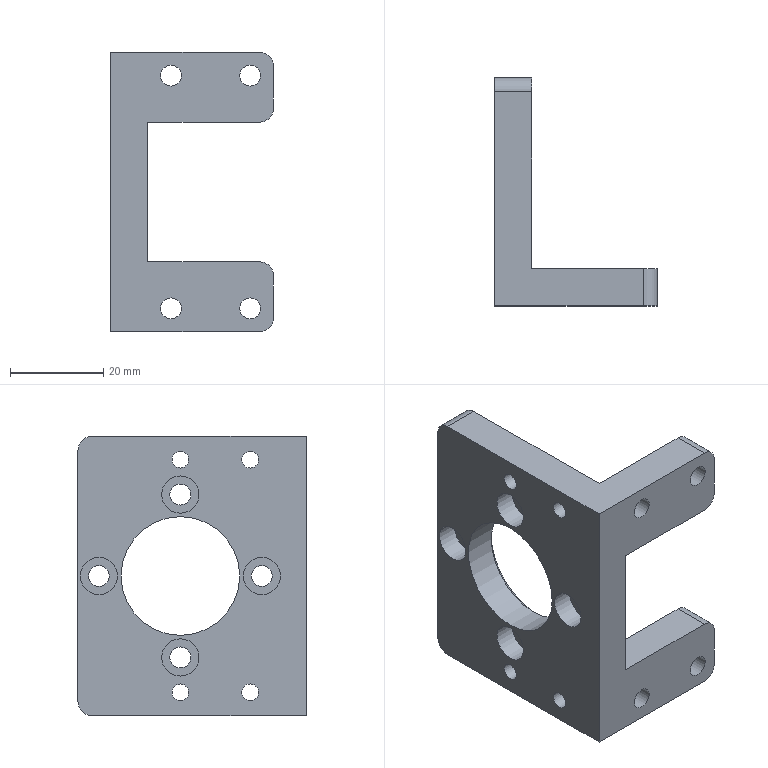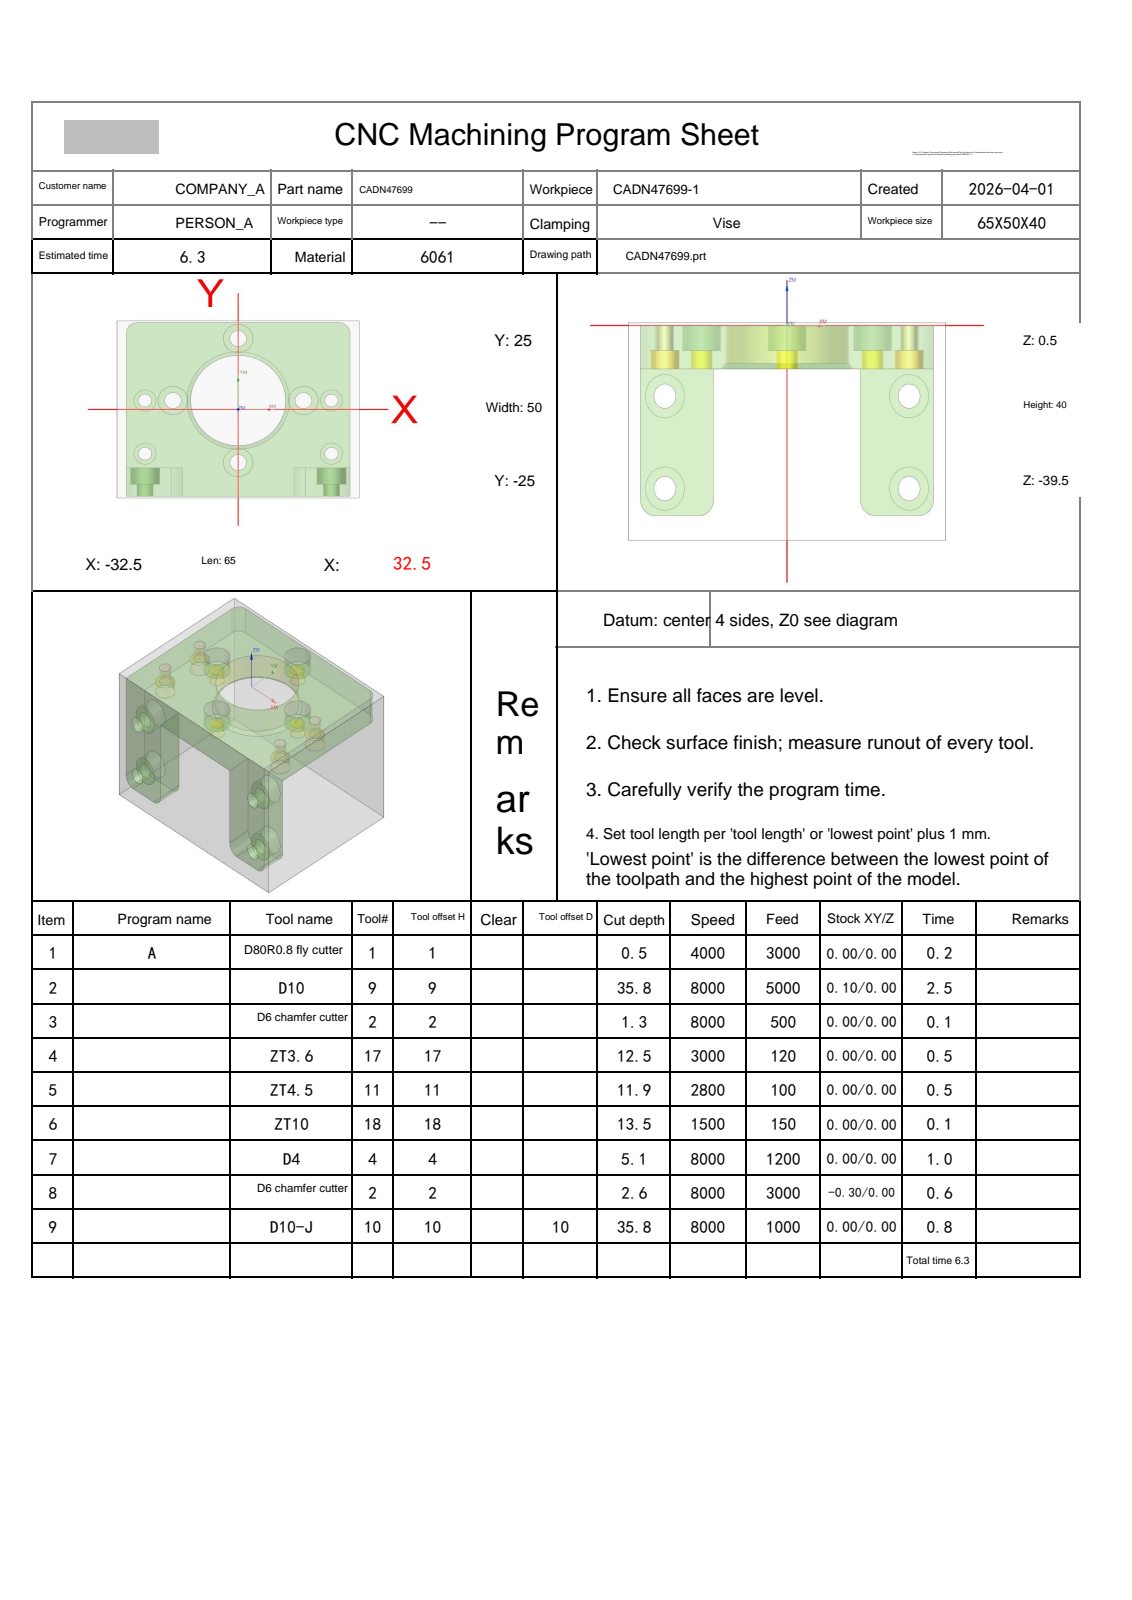NC program | NX | posted by the shop | part box 35 x 49 x 60 mm
Whole program:
%
O0001
(Machine time: 8.03 MIN)
(===Total Tool:8===)
(T1=D80R0.8 fly cutter D=80.  R=0.8  D-  H01 Z=0.    )
(T9=D10     D=10.  R=0.   D-  H09 Z=-35.3 )
(T2=D6 chamfer cutter   D=6.   R=0.   D-  H02 Z=-2.1  )
(T17=ZT3.6  D=3.6  DR_a=118 D-  H17 Z=-12.  )
(T11=ZT4.5  D=4.5  DR_a=118 D-  H11 Z=-11.35)
(T18=ZT10   D=10.  DR_a=118 D-  H18 Z=-13.  )
(T4=D4      D=4.   R=0.   D4  H04 Z=-4.6  )
(T10=D10-J  D=10.  R=0.   D10 H10 Z=-35.3 )
G80 G90 G17 G49 G40
G91 G28 Z0
M01
N1 T01 M06
(D80R0.8 fly cutter  D=80. R=0.8 H=01 ce=0.20 di=0.10)
G00 G90 G54 X-75. Y0.0 M03 S4000
G43 H01 Z20.
M08
Z2.1
G01 Z.1 F3000.
X-70.
X70.
X75.
Z2.1
G00 Z20.
G00 G90 X-75. Y0.0 M03 S4000
Z20.
Z2.
G01 Z0.0 F1000.
X-70.
X70.
X75.
Z2.
G00 Z20.
G91 G28 Z0.0
M05
M09
G91 G28 Z0.0
M01
N2 T09 M06
(D10  D=10. R=0. H=09 ce=0.10 di=0.00)
G00 G90 G54 X0.0 Y-29.6 M03 S8000
G43 H09 Z20.
M08
Z.5
G01 X-30. Z.404 F5000.
G02 X-35.1 Y-24.5 Z.378 I0.0 J5.1
G01 Y21.5 Z.23
G02 X-27. Y29.6 Z.189 I8.1 J0.0
G01 X27. Z.015
G02 X35.1 Y21.5 Z-.025 I0.0 J-8.1
G01 Y-24.5 Z-.173
G02 X30. Y-29.6 Z-.199 I-5.1 J0.0
G01 X-30. Z-.392
G02 X-35.1 Y-24.5 Z-.418 I0.0 J5.1
G01 Y21.5 Z-.566
G02 X-27. Y29.6 Z-.607 I8.1 J0.0
G01 X27. Z-.78
G02 X35.1 Y21.5 Z-.821 I0.0 J-8.1
G01 Y-24.5 Z-.969
G02 X30. Y-29.6 Z-.995 I-5.1 J0.0
G01 X-30. Z-1.188
G02 X-35.1 Y-24.5 Z-1.213 I0.0 J5.1
G01 Y21.5 Z-1.361
G02 X-27. Y29.6 Z-1.402 I8.1 J0.0
G01 X27. Z-1.576
G02 X35.1 Y21.5 Z-1.617 I0.0 J-8.1
G01 Y-24.5 Z-1.764
G02 X30. Y-29.6 Z-1.79 I-5.1 J0.0
G01 X-30. Z-1.983
G02 X-35.1 Y-24.5 Z-2.009 I0.0 J5.1
G01 Y21.5 Z-2.157
G02 X-27. Y29.6 Z-2.198 I8.1 J0.0
G01 X27. Z-2.371
G02 X35.1 Y21.5 Z-2.412 I0.0 J-8.1
G01 Y-24.5 Z-2.56
G02 X30. Y-29.6 Z-2.586 I-5.1 J0.0
G01 X-30. Z-2.779
G02 X-35.1 Y-24.5 Z-2.804 I0.0 J5.1
G01 Y21.5 Z-2.952
G02 X-27. Y29.6 Z-2.993 I8.1 J0.0
G01 X27. Z-3.167
G02 X35.1 Y21.5 Z-3.208 I0.0 J-8.1
G01 Y-24.5 Z-3.356
G02 X30. Y-29.6 Z-3.381 I-5.1 J0.0
G01 X-30. Z-3.574
G02 X-35.1 Y-24.5 Z-3.6 I0.0 J5.1
G01 Y21.5 Z-3.748
G02 X-27. Y29.6 Z-3.789 I8.1 J0.0
G01 X27. Z-3.962
G02 X35.1 Y21.5 Z-4.003 I0.0 J-8.1
G01 Y-24.5 Z-4.151
G02 X30. Y-29.6 Z-4.177 I-5.1 J0.0
G01 X-30. Z-4.37
G02 X-35.1 Y-24.5 Z-4.396 I0.0 J5.1
G01 Y21.5 Z-4.543
G02 X-27. Y29.6 Z-4.584 I8.1 J0.0
G01 X27. Z-4.758
G02 X35.1 Y21.5 Z-4.799 I0.0 J-8.1
G01 Y-24.5 Z-4.947
G02 X30. Y-29.6 Z-4.972 I-5.1 J0.0
G01 X-30. Z-5.165
G02 X-35.1 Y-24.5 Z-5.191 I0.0 J5.1
G01 Y21.5 Z-5.339
G02 X-27. Y29.6 Z-5.38 I8.1 J0.0
G01 X27. Z-5.553
G02 X35.1 Y21.5 Z-5.594 I0.0 J-8.1
G01 Y-24.5 Z-5.742
G02 X30. Y-29.6 Z-5.768 I-5.1 J0.0
G01 X-30. Z-5.961
G02 X-35.1 Y-24.5 Z-5.987 I0.0 J5.1
G01 Y21.5 Z-6.135
G02 X-27. Y29.6 Z-6.175 I8.1 J0.0
G01 X27. Z-6.349
G02 X35.1 Y21.5 Z-6.39 I0.0 J-8.1
G01 Y-24.5 Z-6.538
G02 X30. Y-29.6 Z-6.564 I-5.1 J0.0
G01 X-30. Z-6.756
G02 X-35.1 Y-24.5 Z-6.782 I0.0 J5.1
G01 Y21.5 Z-6.93
G02 X-27. Y29.6 Z-6.971 I8.1 J0.0
G01 X27. Z-7.145
G02 X35.1 Y21.5 Z-7.185 I0.0 J-8.1
G01 Y-24.5 Z-7.333
G02 X30. Y-29.6 Z-7.359 I-5.1 J0.0
G01 X-30. Z-7.552
G02 X-35.1 Y-24.5 Z-7.578 I0.0 J5.1
G01 Y21.5 Z-7.726
G02 X-27. Y29.6 Z-7.767 I8.1 J0.0
G01 X27. Z-7.94
G02 X35.1 Y21.5 Z-7.981 I0.0 J-8.1
G01 Y-24.5 Z-8.129
G02 X30. Y-29.6 Z-8.155 I-5.1 J0.0
G01 X-30. Z-8.348
G02 X-35.1 Y-24.5 Z-8.373 I0.0 J5.1
G01 Y21.5 Z-8.521
G02 X-27. Y29.6 Z-8.562 I8.1 J0.0
G01 X27. Z-8.736
G02 X35.1 Y21.5 Z-8.777 I0.0 J-8.1
G01 Y-24.5 Z-8.924
G02 X30. Y-29.6 Z-8.95 I-5.1 J0.0
G01 X-30. Z-9.143
G02 X-35.1 Y-24.5 Z-9.169 I0.0 J5.1
G01 Y21.5 Z-9.317
G02 X-27. Y29.6 Z-9.358 I8.1 J0.0
G01 X27. Z-9.531
G02 X35.1 Y21.5 Z-9.572 I0.0 J-8.1
G01 Y-24.5 Z-9.72
G02 X30. Y-29.6 Z-9.746 I-5.1 J0.0
G01 X-30. Z-9.939
G02 X-35.1 Y-24.5 Z-9.964 I0.0 J5.1
G01 Y21.5 Z-10.112
G02 X-27. Y29.6 Z-10.153 I8.1 J0.0
G01 X27. Z-10.327
G02 X35.1 Y21.5 Z-10.368 I0.0 J-8.1
G01 Y-24.5 Z-10.516
G02 X30. Y-29.6 Z-10.541 I-5.1 J0.0
G01 X-30. Z-10.734
G02 X-35.1 Y-24.5 Z-10.76 I0.0 J5.1
G01 Y21.5 Z-10.908
G02 X-27. Y29.6 Z-10.949 I8.1 J0.0
G01 X27. Z-11.122
G02 X35.1 Y21.5 Z-11.163 I0.0 J-8.1
G01 Y-24.5 Z-11.311
G02 X30. Y-29.6 Z-11.337 I-5.1 J0.0
G01 X-30. Z-11.53
G02 X-35.1 Y-24.5 Z-11.556 I0.0 J5.1
G01 Y21.5 Z-11.703
G02 X-27. Y29.6 Z-11.744 I8.1 J0.0
G01 X27. Z-11.918
G02 X35.1 Y21.5 Z-11.959 I0.0 J-8.1
G01 Y-24.5 Z-12.107
G02 X30. Y-29.6 Z-12.132 I-5.1 J0.0
G01 X-30. Z-12.325
G02 X-35.1 Y-24.5 Z-12.351 I0.0 J5.1
G01 Y21.5 Z-12.499
G02 X-27. Y29.6 Z-12.54 I8.1 J0.0
G01 X27. Z-12.713
G02 X35.1 Y21.5 Z-12.754 I0.0 J-8.1
G01 Y-24.5 Z-12.902
G02 X30. Y-29.6 Z-12.928 I-5.1 J0.0
G01 X-30. Z-13.121
G02 X-35.1 Y-24.5 Z-13.147 I0.0 J5.1
G01 Y21.5 Z-13.295
G02 X-27. Y29.6 Z-13.335 I8.1 J0.0
G01 X27. Z-13.509
G02 X35.1 Y21.5 Z-13.55 I0.0 J-8.1
G01 Y-24.5 Z-13.698
G02 X30. Y-29.6 Z-13.724 I-5.1 J0.0
G01 X-30. Z-13.916
G02 X-35.1 Y-24.5 Z-13.942 I0.0 J5.1
G01 Y21.5 Z-14.09
G02 X-27. Y29.6 Z-14.131 I8.1 J0.0
G01 X27. Z-14.305
G02 X35.1 Y21.5 Z-14.345 I0.0 J-8.1
G01 Y-24.5 Z-14.493
G02 X30. Y-29.6 Z-14.519 I-5.1 J0.0
G01 X-30. Z-14.712
G02 X-35.1 Y-24.5 Z-14.738 I0.0 J5.1
G01 Y21.5 Z-14.886
G02 X-27. Y29.6 Z-14.927 I8.1 J0.0
G01 X27. Z-15.1
G02 X35.1 Y21.5 Z-15.141 I0.0 J-8.1
G01 Y-24.5 Z-15.289
G02 X30. Y-29.6 Z-15.315 I-5.1 J0.0
G01 X-30. Z-15.508
G02 X-35.1 Y-24.5 Z-15.533 I0.0 J5.1
G01 Y21.5 Z-15.681
G02 X-27. Y29.6 Z-15.722 I8.1 J0.0
G01 X27. Z-15.896
G02 X35.1 Y21.5 Z-15.937 I0.0 J-8.1
G01 Y-24.5 Z-16.084
G02 X30. Y-29.6 Z-16.11 I-5.1 J0.0
G01 X-30. Z-16.303
G02 X-35.1 Y-24.5 Z-16.329 I0.0 J5.1
G01 Y21.5 Z-16.477
G02 X-27. Y29.6 Z-16.518 I8.1 J0.0
G01 X27. Z-16.691
G02 X35.1 Y21.5 Z-16.732 I0.0 J-8.1
G01 Y-24.5 Z-16.88
G02 X30. Y-29.6 Z-16.906 I-5.1 J0.0
G01 X-30. Z-17.099
G02 X-35.1 Y-24.5 Z-17.124 I0.0 J5.1
G01 Y21.5 Z-17.272
G02 X-27. Y29.6 Z-17.313 I8.1 J0.0
G01 X27. Z-17.487
G02 X35.1 Y21.5 Z-17.528 I0.0 J-8.1
G01 Y-24.5 Z-17.676
G02 X30. Y-29.6 Z-17.701 I-5.1 J0.0
G01 X-30. Z-17.894
G02 X-35.1 Y-24.5 Z-17.92 I0.0 J5.1
G01 Y21.5 Z-18.068
G02 X-27. Y29.6 Z-18.109 I8.1 J0.0
G01 X27. Z-18.282
G02 X35.1 Y21.5 Z-18.323 I0.0 J-8.1
G01 Y-24.5 Z-18.471
G02 X30. Y-29.6 Z-18.497 I-5.1 J0.0
G01 X-30. Z-18.69
G02 X-35.1 Y-24.5 Z-18.716 I0.0 J5.1
G01 Y21.5 Z-18.863
G02 X-27. Y29.6 Z-18.904 I8.1 J0.0
G01 X27. Z-19.078
G02 X35.1 Y21.5 Z-19.119 I0.0 J-8.1
G01 Y-24.5 Z-19.267
G02 X30. Y-29.6 Z-19.292 I-5.1 J0.0
G01 X-30. Z-19.485
G02 X-35.1 Y-24.5 Z-19.511 I0.0 J5.1
G01 Y21.5 Z-19.659
G02 X-27. Y29.6 Z-19.7 I8.1 J0.0
G01 X27. Z-19.873
G02 X35.1 Y21.5 Z-19.914 I0.0 J-8.1
G01 Y-24.5 Z-20.062
G02 X30. Y-29.6 Z-20.088 I-5.1 J0.0
G01 X-30. Z-20.281
G02 X-35.1 Y-24.5 Z-20.307 I0.0 J5.1
G01 Y21.5 Z-20.455
G02 X-27. Y29.6 Z-20.495 I8.1 J0.0
G01 X27. Z-20.669
G02 X35.1 Y21.5 Z-20.71 I0.0 J-8.1
G01 Y-24.5 Z-20.858
G02 X30. Y-29.6 Z-20.884 I-5.1 J0.0
G01 X-30. Z-21.076
G02 X-35.1 Y-24.5 Z-21.102 I0.0 J5.1
G01 Y21.5 Z-21.25
G02 X-27. Y29.6 Z-21.291 I8.1 J0.0
G01 X27. Z-21.465
G02 X35.1 Y21.5 Z-21.505 I0.0 J-8.1
G01 Y-24.5 Z-21.653
G02 X30. Y-29.6 Z-21.679 I-5.1 J0.0
G01 X-30. Z-21.872
G02 X-35.1 Y-24.5 Z-21.898 I0.0 J5.1
G01 Y21.5 Z-22.046
G02 X-27. Y29.6 Z-22.087 I8.1 J0.0
G01 X27. Z-22.26
G02 X35.1 Y21.5 Z-22.301 I0.0 J-8.1
G01 Y-24.5 Z-22.449
G02 X30. Y-29.6 Z-22.475 I-5.1 J0.0
G01 X-30. Z-22.668
G02 X-35.1 Y-24.5 Z-22.693 I0.0 J5.1
G01 Y21.5 Z-22.841
G02 X-27. Y29.6 Z-22.882 I8.1 J0.0
G01 X27. Z-23.056
G02 X35.1 Y21.5 Z-23.097 I0.0 J-8.1
G01 Y-24.5 Z-23.244
G02 X30. Y-29.6 Z-23.27 I-5.1 J0.0
G01 X-30. Z-23.463
G02 X-35.1 Y-24.5 Z-23.489 I0.0 J5.1
G01 Y21.5 Z-23.637
G02 X-27. Y29.6 Z-23.678 I8.1 J0.0
G01 X27. Z-23.851
G02 X35.1 Y21.5 Z-23.892 I0.0 J-8.1
G01 Y-24.5 Z-24.04
G02 X30. Y-29.6 Z-24.066 I-5.1 J0.0
G01 X-30. Z-24.259
G02 X-35.1 Y-24.5 Z-24.284 I0.0 J5.1
G01 Y21.5 Z-24.432
G02 X-27. Y29.6 Z-24.473 I8.1 J0.0
G01 X27. Z-24.647
G02 X35.1 Y21.5 Z-24.688 I0.0 J-8.1
G01 Y-24.5 Z-24.836
G02 X30. Y-29.6 Z-24.861 I-5.1 J0.0
G01 X-30. Z-25.054
G02 X-35.1 Y-24.5 Z-25.08 I0.0 J5.1
G01 Y21.5 Z-25.228
G02 X-27. Y29.6 Z-25.269 I8.1 J0.0
G01 X27. Z-25.442
G02 X35.1 Y21.5 Z-25.483 I0.0 J-8.1
G01 Y-24.5 Z-25.631
G02 X30. Y-29.6 Z-25.657 I-5.1 J0.0
G01 X-30. Z-25.85
G02 X-35.1 Y-24.5 Z-25.876 I0.0 J5.1
G01 Y21.5 Z-26.023
G02 X-27. Y29.6 Z-26.064 I8.1 J0.0
G01 X27. Z-26.238
G02 X35.1 Y21.5 Z-26.279 I0.0 J-8.1
G01 Y-24.5 Z-26.427
G02 X30. Y-29.6 Z-26.452 I-5.1 J0.0
G01 X-30. Z-26.645
G02 X-35.1 Y-24.5 Z-26.671 I0.0 J5.1
G01 Y21.5 Z-26.819
G02 X-27. Y29.6 Z-26.86 I8.1 J0.0
G01 X27. Z-27.033
G02 X35.1 Y21.5 Z-27.074 I0.0 J-8.1
G01 Y-24.5 Z-27.222
G02 X30. Y-29.6 Z-27.248 I-5.1 J0.0
G01 X-30. Z-27.441
G02 X-35.1 Y-24.5 Z-27.467 I0.0 J5.1
G01 Y21.5 Z-27.615
G02 X-27. Y29.6 Z-27.655 I8.1 J0.0
G01 X27. Z-27.829
G02 X35.1 Y21.5 Z-27.87 I0.0 J-8.1
G01 Y-24.5 Z-28.018
G02 X30. Y-29.6 Z-28.044 I-5.1 J0.0
G01 X-30. Z-28.236
G02 X-35.1 Y-24.5 Z-28.262 I0.0 J5.1
G01 Y21.5 Z-28.41
G02 X-27. Y29.6 Z-28.451 I8.1 J0.0
G01 X27. Z-28.625
G02 X35.1 Y21.5 Z-28.665 I0.0 J-8.1
G01 Y-24.5 Z-28.813
G02 X30. Y-29.6 Z-28.839 I-5.1 J0.0
G01 X-30. Z-29.032
G02 X-35.1 Y-24.5 Z-29.058 I0.0 J5.1
G01 Y21.5 Z-29.206
G02 X-27. Y29.6 Z-29.247 I8.1 J0.0
G01 X27. Z-29.42
G02 X35.1 Y21.5 Z-29.461 I0.0 J-8.1
G01 Y-24.5 Z-29.609
G02 X30. Y-29.6 Z-29.635 I-5.1 J0.0
G01 X-30. Z-29.828
G02 X-35.1 Y-24.5 Z-29.853 I0.0 J5.1
G01 Y21.5 Z-30.001
G02 X-27. Y29.6 Z-30.042 I8.1 J0.0
G01 X27. Z-30.216
G02 X35.1 Y21.5 Z-30.257 I0.0 J-8.1
G01 Y-24.5 Z-30.404
G02 X30. Y-29.6 Z-30.43 I-5.1 J0.0
G01 X-30. Z-30.623
G02 X-35.1 Y-24.5 Z-30.649 I0.0 J5.1
G01 Y21.5 Z-30.797
G02 X-27. Y29.6 Z-30.838 I8.1 J0.0
G01 X27. Z-31.011
G02 X35.1 Y21.5 Z-31.052 I0.0 J-8.1
G01 Y-24.5 Z-31.2
G02 X30. Y-29.6 Z-31.226 I-5.1 J0.0
G01 X-30. Z-31.419
G02 X-35.1 Y-24.5 Z-31.444 I0.0 J5.1
G01 Y21.5 Z-31.592
G02 X-27. Y29.6 Z-31.633 I8.1 J0.0
G01 X27. Z-31.807
G02 X35.1 Y21.5 Z-31.848 I0.0 J-8.1
G01 Y-24.5 Z-31.996
G02 X30. Y-29.6 Z-32.021 I-5.1 J0.0
G01 X-30. Z-32.214
G02 X-35.1 Y-24.5 Z-32.24 I0.0 J5.1
G01 Y21.5 Z-32.388
G02 X-27. Y29.6 Z-32.429 I8.1 J0.0
G01 X27. Z-32.602
G02 X35.1 Y21.5 Z-32.643 I0.0 J-8.1
G01 Y-24.5 Z-32.791
G02 X30. Y-29.6 Z-32.817 I-5.1 J0.0
G01 X-30. Z-33.01
G02 X-35.1 Y-24.5 Z-33.036 I0.0 J5.1
G01 Y21.5 Z-33.183
G02 X-27. Y29.6 Z-33.224 I8.1 J0.0
G01 X27. Z-33.398
G02 X35.1 Y21.5 Z-33.439 I0.0 J-8.1
G01 Y-24.5 Z-33.587
G02 X30. Y-29.6 Z-33.612 I-5.1 J0.0
G01 X-30. Z-33.805
G02 X-35.1 Y-24.5 Z-33.831 I0.0 J5.1
G01 Y21.5 Z-33.979
G02 X-27. Y29.6 Z-34.02 I8.1 J0.0
G01 X27. Z-34.193
G02 X35.1 Y21.5 Z-34.234 I0.0 J-8.1
G01 Y-24.5 Z-34.382
G02 X30. Y-29.6 Z-34.408 I-5.1 J0.0
G01 X-30. Z-34.601
G02 X-35.1 Y-24.5 Z-34.627 I0.0 J5.1
G01 Y21.5 Z-34.775
G02 X-27. Y29.6 Z-34.815 I8.1 J0.0
G01 X27. Z-34.989
G02 X35.1 Y21.5 Z-35.03 I0.0 J-8.1
G01 Y-24.5 Z-35.178
G02 X30. Y-29.6 Z-35.204 I-5.1 J0.0
G01 X0.0 Z-35.3
X-30.
G02 X-35.1 Y-24.5 I0.0 J5.1
G01 Y21.5
G02 X-27. Y29.6 I8.1 J0.0
G01 X27.
G02 X35.1 Y21.5 I0.0 J-8.1
G01 Y-24.5
G02 X30. Y-29.6 I-5.1 J0.0
G01 X0.0
X-.5
Z-34.3
G00 Z20.
G00 G90 X4.627 Y-3.566 M03 S8000
Z20.
Z1.
G01 X5.431 Y-2.931 Z.946 F4000.
X6.535 Y-1.534 Z.853
X7.288 Y.079 Z.76
X7.65 Y1.822 Z.666
Y3.178 Z.595
X7.288 Y4.921 Z.502
X6.535 Y6.534 Z.409
X5.431 Y7.931 Z.315
X4.034 Y9.035 Z.222
X2.421 Y9.788 Z.129
X.678 Y10.15 Z.036
X0.0 Z0.0
G03 X-7.65 Y2.5 Z-.142 I0.0 J-7.65
X0.0 Y-5.15 Z-.283 I7.65 J0.0
X7.65 Y2.5 Z-.425 I0.0 J7.65
X0.0 Y10.15 Z-.567 I-7.65 J0.0
X-7.65 Y2.5 Z-.708 I0.0 J-7.65
X0.0 Y-5.15 Z-.85 I7.65 J0.0
X7.65 Y2.5 Z-.992 I0.0 J7.65
X0.0 Y10.15 Z-1.133 I-7.65 J0.0
X-7.65 Y2.5 Z-1.275 I0.0 J-7.65
X0.0 Y-5.15 Z-1.417 I7.65 J0.0
X7.65 Y2.5 Z-1.558 I0.0 J7.65
X0.0 Y10.15 Z-1.7 I-7.65 J0.0
X-7.65 Y2.5 Z-1.842 I0.0 J-7.65
X0.0 Y-5.15 Z-1.983 I7.65 J0.0
X7.65 Y2.5 Z-2.125 I0.0 J7.65
X0.0 Y10.15 Z-2.267 I-7.65 J0.0
X-7.65 Y2.5 Z-2.408 I0.0 J-7.65
X0.0 Y-5.15 Z-2.55 I7.65 J0.0
X7.65 Y2.5 Z-2.692 I0.0 J7.65
X0.0 Y10.15 Z-2.833 I-7.65 J0.0
X-7.65 Y2.5 Z-2.975 I0.0 J-7.65
X0.0 Y-5.15 Z-3.117 I7.65 J0.0
X7.65 Y2.5 Z-3.258 I0.0 J7.65
X0.0 Y10.15 Z-3.4 I-7.65 J0.0
X-7.65 Y2.5 Z-3.542 I0.0 J-7.65
X0.0 Y-5.15 Z-3.683 I7.65 J0.0
X7.65 Y2.5 Z-3.825 I0.0 J7.65
X0.0 Y10.15 Z-3.967 I-7.65 J0.0
X-7.65 Y2.5 Z-4.108 I0.0 J-7.65
X0.0 Y-5.15 Z-4.25 I7.65 J0.0
X7.65 Y2.5 Z-4.392 I0.0 J7.65
X0.0 Y10.15 Z-4.533 I-7.65 J0.0
X-7.65 Y2.5 Z-4.675 I0.0 J-7.65
X0.0 Y-5.15 Z-4.817 I7.65 J0.0
X7.65 Y2.5 Z-4.958 I0.0 J7.65
X0.0 Y10.15 Z-5.1 I-7.65 J0.0
X-7.65 Y2.5 Z-5.242 I0.0 J-7.65
X0.0 Y-5.15 Z-5.383 I7.65 J0.0
X7.65 Y2.5 Z-5.525 I0.0 J7.65
X0.0 Y10.15 Z-5.667 I-7.65 J0.0
X-7.65 Y2.5 Z-5.808 I0.0 J-7.65
X0.0 Y-5.15 Z-5.95 I7.65 J0.0
X7.65 Y2.5 Z-6.092 I0.0 J7.65
X0.0 Y10.15 Z-6.233 I-7.65 J0.0
X-7.65 Y2.5 Z-6.375 I0.0 J-7.65
X0.0 Y-5.15 Z-6.517 I7.65 J0.0
X7.65 Y2.5 Z-6.658 I0.0 J7.65
X0.0 Y10.15 Z-6.8 I-7.65 J0.0
X-7.65 Y2.5 Z-6.942 I0.0 J-7.65
X0.0 Y-5.15 Z-7.083 I7.65 J0.0
X7.65 Y2.5 Z-7.225 I0.0 J7.65
X0.0 Y10.15 Z-7.367 I-7.65 J0.0
X-7.65 Y2.5 Z-7.508 I0.0 J-7.65
X0.0 Y-5.15 Z-7.65 I7.65 J0.0
X7.65 Y2.5 Z-7.792 I0.0 J7.65
X0.0 Y10.15 Z-7.933 I-7.65 J0.0
X-7.65 Y2.5 Z-8.075 I0.0 J-7.65
X0.0 Y-5.15 Z-8.217 I7.65 J0.0
X7.65 Y2.5 Z-8.358 I0.0 J7.65
X0.0 Y10.15 Z-8.5 I-7.65 J0.0
X-7.65 Y2.5 I0.0 J-7.65
X0.0 Y-5.15 I7.65 J0.0
X7.65 Y2.5 I0.0 J7.65
X0.0 Y10.15 I-7.65 J0.0
X-.4 Y10.14 I0.0 J-7.65
G01 Z-7.5
G00 Z20.
G91 G28 Z0.0
M05
M09
G91 G28 Z0.0
M01
N3 T02 M06
(D6 chamfer cutter  D=6. R=0. H=02 ce=0.00 di=0.10)
G00 G90 G54 X0.0 Y2.5 M03 S8000
G43 H02 Z20.
M08
G98 G82 X0.0 Y2.5 Z-.8 R1. F500.
G80
G00 Z20.
G00 G90 X0.0 Y20. M03 S8000
Z20.
G98 G81 X0.0 Y20. Z-.8 R1. F500.
X17.5 Y2.5
X25.
Y-12.5
X0.0 Y-15.
X-17.5 Y2.5
X-25.
Y-12.5
G80
G00 Z20.
G91 G28 Z0.0
M05
M09
G91 G28 Z0.0
M01
N4 T17 M06
(ZT3.6 D=3.6 DR_a=118 H=17)
G00 G90 G54 X-25. Y2.5 M03 S3000
G43 H17 Z20.
M08
G98 G83 X-25. Y2.5 Z-12. R1. F120. Q3.
Y-12.5
X25.
Y2.5
G80
G00 Z20.
G91 G28 Z0.0
M05
M09
G91 G28 Z0.0
M01
N5 T11 M06
(ZT4.5 D=4.5 DR_a=118 H=11)
G00 G90 G54 X0.0 Y20. M03 S2800
G43 H11 Z20.
M08
G98 G83 X0.0 Y20. Z-11.352 R1. F100. Q2.
X-17.5 Y2.5
X0.0 Y-15.
X17.5 Y2.5
G80
G00 Z20.
G91 G28 Z0.0
M05
M09
G91 G28 Z0.0
M01
N6 T18 M06
(ZT10 D=10. DR_a=118 H=18)
G00 G90 G54 X0.0 Y2.5 M03 S1500
G43 H18 Z20.
M08
G98 G83 X0.0 Y2.5 Z-13.004 R1. F150. Q3.
G80
G00 Z20.
G91 G28 Z0.0
M05
M09
G91 G28 Z0.0
M01
N7 T04 M06
(D4  D=4. R=0. H=04 ce=0.10 di=0.00)
G00 G90 G54 X0.0 Y-15. M03 S8000
G43 H04 Z20.
M08
Z.5
G03 X.95 Y-14.05 I0.0 J.95 F1200.
X0.0 Y-13.1 I-.95 J0.0
X0.0 Y-13.1 Z.2 I0.0 J-1.9
X0.0 Y-13.1 Z-.1 I0.0 J-1.9
X0.0 Y-13.1 Z-.4 I0.0 J-1.9
X0.0 Y-13.1 Z-.7 I0.0 J-1.9
X0.0 Y-13.1 Z-1. I0.0 J-1.9
X0.0 Y-13.1 Z-1.3 I0.0 J-1.9
X0.0 Y-13.1 Z-1.6 I0.0 J-1.9
X0.0 Y-13.1 Z-1.9 I0.0 J-1.9
X0.0 Y-13.1 Z-2.2 I0.0 J-1.9
X0.0 Y-13.1 Z-2.5 I0.0 J-1.9
X0.0 Y-13.1 Z-2.8 I0.0 J-1.9
X0.0 Y-13.1 Z-3.1 I0.0 J-1.9
X0.0 Y-13.1 Z-3.4 I0.0 J-1.9
X0.0 Y-13.1 Z-3.7 I0.0 J-1.9
X0.0 Y-13.1 Z-4. I0.0 J-1.9
X0.0 Y-13.1 Z-4.3 I0.0 J-1.9
X0.0 Y-13.1 Z-4.6 I0.0 J-1.9
X-1.9 Y-15. I0.0 J-1.9
X0.0 Y-16.9 I1.9 J0.0
X1.9 Y-15. I0.0 J1.9
X0.0 Y-13.1 I-1.9 J0.0
X-.95 Y-14.05 I0.0 J-.95
X0.0 Y-15. I.95 J0.0
G00 Z20.
X-17.5 Y2.5
Z.5
G03 X-16.55 Y3.45 I0.0 J.95
X-17.5 Y4.4 I-.95 J0.0
X-17.5 Y4.4 Z.2 I0.0 J-1.9
X-17.5 Y4.4 Z-.1 I0.0 J-1.9
X-17.5 Y4.4 Z-.4 I0.0 J-1.9
X-17.5 Y4.4 Z-.7 I0.0 J-1.9
X-17.5 Y4.4 Z-1. I0.0 J-1.9
X-17.5 Y4.4 Z-1.3 I0.0 J-1.9
X-17.5 Y4.4 Z-1.6 I0.0 J-1.9
X-17.5 Y4.4 Z-1.9 I0.0 J-1.9
X-17.5 Y4.4 Z-2.2 I0.0 J-1.9
X-17.5 Y4.4 Z-2.5 I0.0 J-1.9
X-17.5 Y4.4 Z-2.8 I0.0 J-1.9
X-17.5 Y4.4 Z-3.1 I0.0 J-1.9
X-17.5 Y4.4 Z-3.4 I0.0 J-1.9
X-17.5 Y4.4 Z-3.7 I0.0 J-1.9
X-17.5 Y4.4 Z-4. I0.0 J-1.9
X-17.5 Y4.4 Z-4.3 I0.0 J-1.9
X-17.5 Y4.4 Z-4.6 I0.0 J-1.9
X-19.4 Y2.5 I0.0 J-1.9
X-17.5 Y.6 I1.9 J0.0
X-15.6 Y2.5 I0.0 J1.9
X-17.5 Y4.4 I-1.9 J0.0
X-18.45 Y3.45 I0.0 J-.95
X-17.5 Y2.5 I.95 J0.0
G00 Z20.
X0.0 Y20.
Z.5
G03 X.95 Y20.95 I0.0 J.95
X0.0 Y21.9 I-.95 J0.0
X0.0 Y21.9 Z.2 I0.0 J-1.9
X0.0 Y21.9 Z-.1 I0.0 J-1.9
X0.0 Y21.9 Z-.4 I0.0 J-1.9
X0.0 Y21.9 Z-.7 I0.0 J-1.9
X0.0 Y21.9 Z-1. I0.0 J-1.9
X0.0 Y21.9 Z-1.3 I0.0 J-1.9
X0.0 Y21.9 Z-1.6 I0.0 J-1.9
X0.0 Y21.9 Z-1.9 I0.0 J-1.9
X0.0 Y21.9 Z-2.2 I0.0 J-1.9
X0.0 Y21.9 Z-2.5 I0.0 J-1.9
X0.0 Y21.9 Z-2.8 I0.0 J-1.9
X0.0 Y21.9 Z-3.1 I0.0 J-1.9
X0.0 Y21.9 Z-3.4 I0.0 J-1.9
X0.0 Y21.9 Z-3.7 I0.0 J-1.9
X0.0 Y21.9 Z-4. I0.0 J-1.9
X0.0 Y21.9 Z-4.3 I0.0 J-1.9
X0.0 Y21.9 Z-4.6 I0.0 J-1.9
X-1.9 Y20. I0.0 J-1.9
X0.0 Y18.1 I1.9 J0.0
X1.9 Y20. I0.0 J1.9
X0.0 Y21.9 I-1.9 J0.0
X-.95 Y20.95 I0.0 J-.95
X0.0 Y20. I.95 J0.0
G00 Z20.
X17.5 Y2.5
Z.5
G03 X18.45 Y3.45 I0.0 J.95
X17.5 Y4.4 I-.95 J0.0
X17.5 Y4.4 Z.2 I0.0 J-1.9
X17.5 Y4.4 Z-.1 I0.0 J-1.9
X17.5 Y4.4 Z-.4 I0.0 J-1.9
X17.5 Y4.4 Z-.7 I0.0 J-1.9
X17.5 Y4.4 Z-1. I0.0 J-1.9
X17.5 Y4.4 Z-1.3 I0.0 J-1.9
X17.5 Y4.4 Z-1.6 I0.0 J-1.9
X17.5 Y4.4 Z-1.9 I0.0 J-1.9
X17.5 Y4.4 Z-2.2 I0.0 J-1.9
X17.5 Y4.4 Z-2.5 I0.0 J-1.9
X17.5 Y4.4 Z-2.8 I0.0 J-1.9
X17.5 Y4.4 Z-3.1 I0.0 J-1.9
X17.5 Y4.4 Z-3.4 I0.0 J-1.9
X17.5 Y4.4 Z-3.7 I0.0 J-1.9
X17.5 Y4.4 Z-4. I0.0 J-1.9
X17.5 Y4.4 Z-4.3 I0.0 J-1.9
X17.5 Y4.4 Z-4.6 I0.0 J-1.9
X15.6 Y2.5 I0.0 J-1.9
X17.5 Y.6 I1.9 J0.0
X19.4 Y2.5 I0.0 J1.9
X17.5 Y4.4 I-1.9 J0.0
X16.55 Y3.45 I0.0 J-.95
X17.5 Y2.5 I.95 J0.0
G00 Z20.
G00 G90 X0.0 Y-15. M03 S8000
Z20.
Z.5
G41 D04
G01 X.196 Y-14.96 F500.
G03 X.99 Y-13.99 I-.196 J.97
X0.0 Y-13. I-.99 J0.0
X0.0 Y-13. Z-4.5 I0.0 J-2.
X-.251 Y-13.016 Z-4.6 I0.0 J-2.
X-2. Y-15. I.251 J-1.984
X0.0 Y-17. I2. J0.0
X2. Y-15. I0.0 J2.
X0.0 Y-13. I-2. J0.0
X-.251 Y-13.016 I0.0 J-2.
X-1.117 Y-13.998 I.124 J-.982
X-.199 Y-14.985 I.99 J0.0
G01 G40 X0.0 Y-15.
G00 Z20.
X-17.5 Y2.5
Z.5
G41 D04
G01 X-17.304 Y2.54
G03 X-16.51 Y3.51 I-.196 J.97
X-17.5 Y4.5 I-.99 J0.0
X-17.5 Y4.5 Z-4.5 I0.0 J-2.
X-17.751 Y4.484 Z-4.6 I0.0 J-2.
X-19.5 Y2.5 I.251 J-1.984
X-17.5 Y.5 I2. J0.0
X-15.5 Y2.5 I0.0 J2.
X-17.5 Y4.5 I-2. J0.0
X-17.751 Y4.484 I0.0 J-2.
X-18.617 Y3.502 I.124 J-.982
X-17.699 Y2.515 I.99 J0.0
G01 G40 X-17.5 Y2.5
G00 Z20.
X0.0 Y20.
Z.5
G41 D04
G01 X.196 Y20.04
G03 X.99 Y21.01 I-.196 J.97
X0.0 Y22. I-.99 J0.0
X0.0 Y22. Z-4.5 I0.0 J-2.
X-.251 Y21.984 Z-4.6 I0.0 J-2.
X-2. Y20. I.251 J-1.984
X0.0 Y18. I2. J0.0
X2. Y20. I0.0 J2.
X0.0 Y22. I-2. J0.0
X-.251 Y21.984 I0.0 J-2.
X-1.117 Y21.002 I.124 J-.982
X-.199 Y20.015 I.99 J0.0
G01 G40 X0.0 Y20.
G00 Z20.
X17.5 Y2.5
Z.5
G41 D04
G01 X17.696 Y2.54
G03 X18.49 Y3.51 I-.196 J.97
X17.5 Y4.5 I-.99 J0.0
X17.5 Y4.5 Z-4.5 I0.0 J-2.
X17.249 Y4.484 Z-4.6 I0.0 J-2.
X15.5 Y2.5 I.251 J-1.984
X17.5 Y.5 I2. J0.0
X19.5 Y2.5 I0.0 J2.
X17.5 Y4.5 I-2. J0.0
X17.249 Y4.484 I0.0 J-2.
X16.383 Y3.502 I.124 J-.982
X17.301 Y2.515 I.99 J0.0
G01 G40 X17.5 Y2.5
G00 Z20.
G91 G28 Z0.0
M05
M09
G91 G28 Z0.0
M01
N8 T02 M06
(D6 chamfer cutter  D=6. R=0. H=02 ce=0.00 di=0.00)
G00 G90 G54 X.25 Y-26.628 M03 S8000
G43 H02 Z20.
M08
Z2.099
G01 Z-1.5 F3000.
G03 X.33 Y-26.328 I-.52 J.3
X.03 Y-25.808 I-.6 J0.0
G01 X0.0 Y-25.8
X-30.
G02 X-31.3 Y-24.5 I0.0 J1.3
G01 Y21.5
G02 X-27. Y25.8 I4.3 J0.0
G01 X27.
G02 X31.3 Y21.5 I0.0 J-4.3
G01 Y-24.5
G02 X30. Y-25.8 I-1.3 J0.0
G01 X0.0
X-.03 Y-25.808
G03 X-.33 Y-26.328 I.3 J-.52
X-.25 Y-26.628 I.6 J0.0
G01 Z2.099
G00 Z20.
X-10.633 Y2.783
Z2.123
G01 Z-1.5
G03 X-10.912 Y2.851 I-.279 J-.531
X-11.443 Y2.53 I0.0 J-.6
G01 X-11.45 Y2.5
G03 X0.0 Y-8.95 I11.45 J0.0
X11.45 Y2.5 I0.0 J11.45
X0.0 Y13.95 I-11.45 J0.0
X-11.45 Y2.5 I0.0 J-11.45
G01 X-11.443 Y2.47
G03 X-10.912 Y2.149 I.531 J.279
X-10.633 Y2.217 I0.0 J.6
G01 Z2.123
G00 Z20.
G00 G90 X-25. Y2.5 M03 S8000
Z20.
G98 G81 X-25. Y2.5 Z-2.1 R3. F500.
Y-12.5
X25.
Y2.5
G80
G00 Z20.
G00 G90 X14.288 Y1.753 M03 S8000
Z20.
Z2.5
G01 X14.34 Y1.538 Z2.42 F500.
X14.476 Y1.172 Z2.278
X14.653 Y.825 Z2.136
X14.871 Y.501 Z1.994
X15.125 Y.205 Z1.852
X15.412 Y-.059 Z1.71
X15.728 Y-.288 Z1.568
X15.972 Y-.428 Z1.465
X16.328 Y-.588 Z1.323
X16.7 Y-.705 Z1.181
X17.084 Y-.777 Z1.039
X17.473 Y-.803 Z.897
X17.862 Y-.783 Z.755
X18.247 Y-.717 Z.613
X18.621 Y-.607 Z.471
X18.98 Y-.453 Z.329
X19.318 Y-.258 Z.187
X19.63 Y-.024 Z.045
X19.913 Y.244 Z-.097
X20.162 Y.545 Z-.239
X20.374 Y.872 Z-.381
X20.546 Y1.222 Z-.523
X20.675 Y1.59 Z-.665
X20.76 Y1.971 Z-.807
X20.8 Y2.359 Z-.949
Y2.5 Z-1.
G03 X17.5 Y5.8 I-3.3 J0.0
X14.2 Y2.5 I0.0 J-3.3
X17.5 Y-.8 I3.3 J0.0
X20.8 Y2.5 I0.0 J3.3
X20.762 Y2.998 I-3.3 J0.0
G01 Z1.5
G00 Z20.
X-3.212 Y19.253
Z2.5
G01 X-3.16 Y19.038 Z2.42
X-3.024 Y18.672 Z2.278
X-2.847 Y18.325 Z2.136
X-2.629 Y18.001 Z1.994
X-2.375 Y17.705 Z1.852
X-2.088 Y17.441 Z1.71
X-1.772 Y17.212 Z1.568
X-1.528 Y17.072 Z1.465
X-1.172 Y16.912 Z1.323
X-.8 Y16.795 Z1.181
X-.416 Y16.723 Z1.039
X-.027 Y16.697 Z.897
X.362 Y16.717 Z.755
X.747 Y16.783 Z.613
X1.121 Y16.893 Z.471
X1.48 Y17.047 Z.329
X1.818 Y17.242 Z.187
X2.13 Y17.476 Z.045
X2.413 Y17.744 Z-.097
X2.662 Y18.045 Z-.239
X2.874 Y18.372 Z-.381
X3.046 Y18.722 Z-.523
X3.175 Y19.09 Z-.665
X3.26 Y19.471 Z-.807
X3.3 Y19.859 Z-.949
Y20. Z-1.
G03 X0.0 Y23.3 I-3.3 J0.0
X-3.3 Y20. I0.0 J-3.3
X0.0 Y16.7 I3.3 J0.0
X3.3 Y20. I0.0 J3.3
X3.262 Y20.498 I-3.3 J0.0
G01 Z1.5
G00 Z20.
X-20.712 Y1.753
Z2.5
G01 X-20.66 Y1.538 Z2.42
X-20.524 Y1.172 Z2.278
X-20.347 Y.825 Z2.136
X-20.129 Y.501 Z1.994
X-19.875 Y.205 Z1.852
X-19.588 Y-.059 Z1.71
X-19.272 Y-.288 Z1.568
X-19.028 Y-.428 Z1.465
X-18.672 Y-.588 Z1.323
X-18.3 Y-.705 Z1.181
X-17.916 Y-.777 Z1.039
X-17.527 Y-.803 Z.897
X-17.138 Y-.783 Z.755
X-16.753 Y-.717 Z.613
X-16.379 Y-.607 Z.471
X-16.02 Y-.453 Z.329
X-15.682 Y-.258 Z.187
X-15.37 Y-.024 Z.045
X-15.087 Y.244 Z-.097
X-14.838 Y.545 Z-.239
X-14.626 Y.872 Z-.381
X-14.454 Y1.222 Z-.523
X-14.325 Y1.59 Z-.665
X-14.24 Y1.971 Z-.807
X-14.2 Y2.359 Z-.949
Y2.5 Z-1.
G03 X-17.5 Y5.8 I-3.3 J0.0
X-20.8 Y2.5 I0.0 J-3.3
X-17.5 Y-.8 I3.3 J0.0
X-14.2 Y2.5 I0.0 J3.3
X-14.238 Y2.998 I-3.3 J0.0
G01 Z1.5
G00 Z20.
X-3.212 Y-15.747
Z2.5
G01 X-3.16 Y-15.962 Z2.42
X-3.024 Y-16.328 Z2.278
X-2.847 Y-16.675 Z2.136
X-2.629 Y-16.999 Z1.994
X-2.375 Y-17.295 Z1.852
X-2.088 Y-17.559 Z1.71
X-1.772 Y-17.788 Z1.568
X-1.528 Y-17.928 Z1.465
X-1.172 Y-18.088 Z1.323
X-.8 Y-18.205 Z1.181
X-.416 Y-18.277 Z1.039
X-.027 Y-18.303 Z.897
X.362 Y-18.283 Z.755
X.747 Y-18.217 Z.613
X1.121 Y-18.107 Z.471
X1.48 Y-17.953 Z.329
X1.818 Y-17.758 Z.187
X2.13 Y-17.524 Z.045
X2.413 Y-17.256 Z-.097
X2.662 Y-16.955 Z-.239
X2.874 Y-16.628 Z-.381
X3.046 Y-16.278 Z-.523
X3.175 Y-15.91 Z-.665
X3.26 Y-15.529 Z-.807
X3.3 Y-15.141 Z-.949
Y-15. Z-1.
G03 X0.0 Y-11.7 I-3.3 J0.0
X-3.3 Y-15. I0.0 J-3.3
X0.0 Y-18.3 I3.3 J0.0
X3.3 Y-15. I0.0 J3.3
X3.262 Y-14.502 I-3.3 J0.0
G01 Z1.5
G00 Z20.
G00 G90 X-9.05 Y5.5 M03 S8000
Z20.
Z-.5
G01 Z-1. F800.
G03 X-12.05 Y2.5 I0.0 J-3.
X0.0 Y-9.55 I12.05 J0.0
X12.05 Y2.5 I0.0 J12.05
X0.0 Y14.55 I-12.05 J0.0
X-12.05 Y2.5 I0.0 J-12.05
X-9.05 Y-.5 I3. J0.0
G01 Z-.5
G00 Z20.
G91 G28 Z0.0
M05
M09
G91 G28 Z0.0
M01
N9 T10 M06
(D10-J  D=10. R=0. H=10 ce=0.00 di=0.00)
G00 G90 G54 X1.5 Y8.367 M03 S8000
G43 H10 Z10.5
M08
Z-6.8
G01 Z-8.3 F1000.
G41 D10
Y8.75
G03 X0.0 Y10.25 I-1.5 J0.0
X-7.75 Y2.5 I0.0 J-7.75
X0.0 Y-5.25 I7.75 J0.0
X7.75 Y2.5 I0.0 J7.75
X0.0 Y10.25 I-7.75 J0.0
X-.4 Y10.24 I0.0 J-7.75
X-1.822 Y8.742 I.077 J-1.498
G01 X-1.82 Y8.664
X-1.811 Y8.482
G40 X-1.801 Y8.282
Z-6.8
G00 Z10.5
G00 G90 X31.013 Y-30.616 M03 S8000
Z20.
Z-11.267
G01 Z-11.767 F1000.
G41 D10
X30.997 Y-30.417
G03 X30. Y-29.5 I-.997 J-.083
G01 X-30.
G02 X-35. Y-24.5 I0.0 J5.
G01 Y21.5
G02 X-27. Y29.5 I8. J0.0
G01 X27.
G02 X35. Y21.5 I0.0 J-8.
G01 Y-24.5
G02 X30. Y-29.5 I-5. J0.0
G01 X29.5
G03 X28.5 Y-30.5 I0.0 J-1.
G01 G40 Y-30.7
Z-11.267
G00 Z20.
X31.013 Y-30.616
Z-23.033
G01 Z-23.533
G41 D10
X30.997 Y-30.417
G03 X30. Y-29.5 I-.997 J-.083
G01 X-30.
G02 X-35. Y-24.5 I0.0 J5.
G01 Y21.5
G02 X-27. Y29.5 I8. J0.0
G01 X27.
G02 X35. Y21.5 I0.0 J-8.
G01 Y-24.5
G02 X30. Y-29.5 I-5. J0.0
G01 X29.5
G03 X28.5 Y-30.5 I0.0 J-1.
G01 G40 Y-30.7
Z-23.033
G00 Z20.
X31.013 Y-30.616
Z-34.8
G01 Z-35.3
G41 D10
X30.997 Y-30.417
G03 X30. Y-29.5 I-.997 J-.083
G01 X-30.
G02 X-35. Y-24.5 I0.0 J5.
G01 Y21.5
G02 X-27. Y29.5 I8. J0.0
G01 X27.
G02 X35. Y21.5 I0.0 J-8.
G01 Y-24.5
G02 X30. Y-29.5 I-5. J0.0
G01 X29.5
G03 X28.5 Y-30.5 I0.0 J-1.
G01 G40 Y-30.7
Z-34.8
G00 Z20.
M05
M09
G91 G28 Z0.0
G91 G28 Y0.0
M30
%